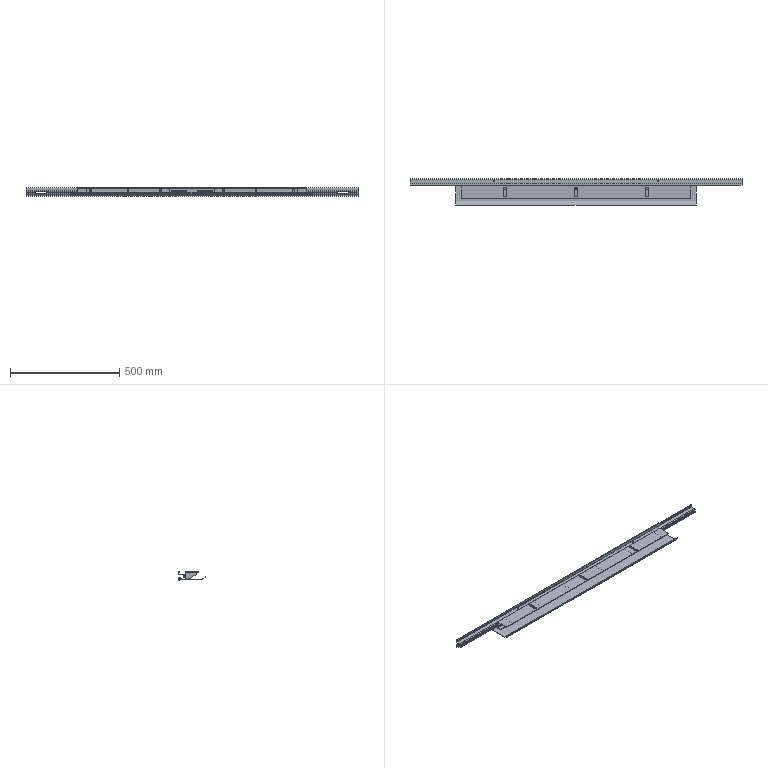Part | SolidWorks | features InContextFeatHolder 2 | 9 solids | 263 faces | box 1520 x 122.321 x 40 mm | volume 769307 mm3 | plane 171 | cylinder 92 | commonest cylinder face diameters 9 x30 6 x25 10 x18 2 x9 12 x4 3 x2